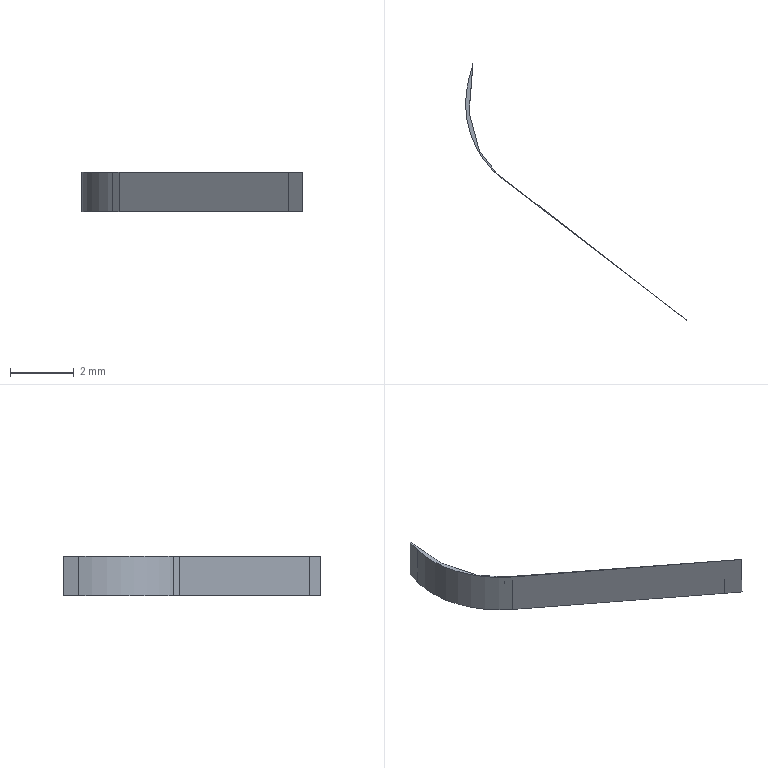Part | STEP file | gslz 2016.10.28-13_id1170_x_t | 1 solid | 10 faces | box 6.934 x 8.042 x 1.25 mm | volume 0.6004 mm3 | plane 9 | cylinder 1 | commonest cylinder face diameters 6 x1
STEP:
#1=CARTESIAN_POINT('',(0.,0.,0.));
#2=DIRECTION('',(0.,0.,1.));
#3=DIRECTION('',(1.,0.,0.));
#4=AXIS2_PLACEMENT_3D('',#1,#2,#3);
#5=CARTESIAN_POINT('',(-225.975,5.758,1.25));
#6=VERTEX_POINT('',#5);
#7=CARTESIAN_POINT('',(-225.435,5.068,1.25));
#8=VERTEX_POINT('',#7);
#9=CARTESIAN_POINT('',(-395.735,222.659,1.25));
#10=DIRECTION('',(0.6163,-0.7875,0.));
#11=VECTOR('',#10,1.);
#12=LINE('',#9,#11);
#13=CARTESIAN_POINT('',(-225.975,5.758,3.25));
#14=DIRECTION('',(0.7875,0.6163,0.));
#15=DIRECTION('',(-0.6163,0.7875,0.));
#16=AXIS2_PLACEMENT_3D('',#13,#14,#15);
#17=PLANE('',#16);
#18=CARTESIAN_POINT('',(275.435,-2.));
#19=DIRECTION('',(-1.,0.));
#20=VECTOR('',#19,1.);
#21=LINE('',#18,#20);
#22=(GEOMETRIC_REPRESENTATION_CONTEXT(2)PARAMETRIC_REPRESENTATION_CONTEXT()REPRESENTATION_CONTEXT('',''));
#23=DEFINITIONAL_REPRESENTATION('',(#21),#22);
#24=PCURVE('',#17,#23);
#25=CARTESIAN_POINT('',(-346.108,261.5,1.25));
#26=DIRECTION('',(0.,0.,-1.));
#27=DIRECTION('',(-1.,0.,0.));
#28=AXIS2_PLACEMENT_3D('',#25,#26,#27);
#29=PLANE('',#28);
#30=CARTESIAN_POINT('',(49.627,-38.841));
#31=DIRECTION('',(-0.6163,-0.7875));
#32=VECTOR('',#31,1.);
#33=LINE('',#30,#32);
#34=(GEOMETRIC_REPRESENTATION_CONTEXT(2)PARAMETRIC_REPRESENTATION_CONTEXT()REPRESENTATION_CONTEXT('',''));
#35=DEFINITIONAL_REPRESENTATION('',(#33),#34);
#36=PCURVE('',#29,#35);
#37=SURFACE_CURVE('',#12,(#24,#36),.PCURVE_S1.);
#38=EDGE_CURVE('',#6,#8,#37,.T.);
#39=ORIENTED_EDGE('',*,*,#38,.T.);
#40=CARTESIAN_POINT('',(-225.435,5.068,0.));
#41=VERTEX_POINT('',#40);
#42=CARTESIAN_POINT('',(-225.435,5.068,3.25));
#43=DIRECTION('',(0.,0.,1.));
#44=VECTOR('',#43,1.);
#45=LINE('',#42,#44);
#46=CARTESIAN_POINT('',(-0.8762,0.));
#47=DIRECTION('',(0.,1.));
#48=VECTOR('',#47,1.);
#49=LINE('',#46,#48);
#50=(GEOMETRIC_REPRESENTATION_CONTEXT(2)PARAMETRIC_REPRESENTATION_CONTEXT()REPRESENTATION_CONTEXT('',''));
#51=DEFINITIONAL_REPRESENTATION('',(#49),#50);
#52=PCURVE('',#17,#51);
#53=CARTESIAN_POINT('',(-225.435,5.068,3.25));
#54=DIRECTION('',(0.6121,0.7907,0.));
#55=DIRECTION('',(-0.7907,0.6121,0.));
#56=AXIS2_PLACEMENT_3D('',#53,#54,#55);
#57=PLANE('',#56);
#58=CARTESIAN_POINT('',(0.,0.));
#59=DIRECTION('',(0.,1.));
#60=VECTOR('',#59,1.);
#61=LINE('',#58,#60);
#62=(GEOMETRIC_REPRESENTATION_CONTEXT(2)PARAMETRIC_REPRESENTATION_CONTEXT()REPRESENTATION_CONTEXT('',''));
#63=DEFINITIONAL_REPRESENTATION('',(#61),#62);
#64=PCURVE('',#57,#63);
#65=SURFACE_CURVE('',#45,(#52,#64),.PCURVE_S1.);
#66=EDGE_CURVE('',#41,#8,#65,.T.);
#67=ORIENTED_EDGE('',*,*,#66,.F.);
#68=CARTESIAN_POINT('',(-225.975,5.758,0.));
#69=VERTEX_POINT('',#68);
#70=CARTESIAN_POINT('',(-225.975,5.758,0.));
#71=DIRECTION('',(0.6163,-0.7875,0.));
#72=VECTOR('',#71,1.);
#73=LINE('',#70,#72);
#74=CARTESIAN_POINT('',(0.,-3.25));
#75=DIRECTION('',(-1.,0.));
#76=VECTOR('',#75,1.);
#77=LINE('',#74,#76);
#78=(GEOMETRIC_REPRESENTATION_CONTEXT(2)PARAMETRIC_REPRESENTATION_CONTEXT()REPRESENTATION_CONTEXT('',''));
#79=DEFINITIONAL_REPRESENTATION('',(#77),#78);
#80=PCURVE('',#17,#79);
#81=CARTESIAN_POINT('',(-346.108,261.5,0.));
#82=DIRECTION('',(0.,0.,-1.));
#83=DIRECTION('',(-1.,0.,0.));
#84=AXIS2_PLACEMENT_3D('',#81,#82,#83);
#85=PLANE('',#84);
#86=CARTESIAN_POINT('',(-120.133,-255.742));
#87=DIRECTION('',(-0.6163,-0.7875));
#88=VECTOR('',#87,1.);
#89=LINE('',#86,#88);
#90=(GEOMETRIC_REPRESENTATION_CONTEXT(2)PARAMETRIC_REPRESENTATION_CONTEXT()REPRESENTATION_CONTEXT('',''));
#91=DEFINITIONAL_REPRESENTATION('',(#89),#90);
#92=PCURVE('',#85,#91);
#93=SURFACE_CURVE('',#73,(#80,#92),.PCURVE_S1.);
#94=EDGE_CURVE('',#69,#41,#93,.T.);
#95=ORIENTED_EDGE('',*,*,#94,.F.);
#96=CARTESIAN_POINT('',(-225.975,5.758,3.25));
#97=DIRECTION('',(0.,0.,1.));
#98=VECTOR('',#97,1.);
#99=LINE('',#96,#98);
#100=CARTESIAN_POINT('',(0.,0.));
#101=DIRECTION('',(0.,1.));
#102=VECTOR('',#101,1.);
#103=LINE('',#100,#102);
#104=(GEOMETRIC_REPRESENTATION_CONTEXT(2)PARAMETRIC_REPRESENTATION_CONTEXT()REPRESENTATION_CONTEXT('',''));
#105=DEFINITIONAL_REPRESENTATION('',(#103),#104);
#106=PCURVE('',#17,#105);
#107=CARTESIAN_POINT('',(-226.305,6.991,3.25));
#108=DIRECTION('',(0.966,0.2585,0.));
#109=DIRECTION('',(-0.2585,0.966,0.));
#110=AXIS2_PLACEMENT_3D('',#107,#108,#109);
#111=PLANE('',#110);
#112=CARTESIAN_POINT('',(-1.276,0.));
#113=DIRECTION('',(0.,1.));
#114=VECTOR('',#113,1.);
#115=LINE('',#112,#114);
#116=(GEOMETRIC_REPRESENTATION_CONTEXT(2)PARAMETRIC_REPRESENTATION_CONTEXT()REPRESENTATION_CONTEXT('',''));
#117=DEFINITIONAL_REPRESENTATION('',(#115),#116);
#118=PCURVE('',#111,#117);
#119=SURFACE_CURVE('',#99,(#106,#118),.PCURVE_S1.);
#120=EDGE_CURVE('',#69,#6,#119,.T.);
#121=ORIENTED_EDGE('',*,*,#120,.T.);
#122=EDGE_LOOP('',(#39,#67,#95,#121));
#123=FACE_BOUND('',#122,.T.);
#124=ADVANCED_FACE('',(#123),#17,.T.);
#125=CARTESIAN_POINT('',(-226.305,6.991,1.25));
#126=VERTEX_POINT('',#125);
#127=CARTESIAN_POINT('',(-297.867,274.409,1.25));
#128=DIRECTION('',(0.2585,-0.966,0.));
#129=VECTOR('',#128,1.);
#130=LINE('',#127,#129);
#131=CARTESIAN_POINT('',(276.828,-2.));
#132=DIRECTION('',(-1.,0.));
#133=VECTOR('',#132,1.);
#134=LINE('',#131,#133);
#135=(GEOMETRIC_REPRESENTATION_CONTEXT(2)PARAMETRIC_REPRESENTATION_CONTEXT()REPRESENTATION_CONTEXT('',''));
#136=DEFINITIONAL_REPRESENTATION('',(#134),#135);
#137=PCURVE('',#111,#136);
#138=CARTESIAN_POINT('',(-48.241,12.909));
#139=DIRECTION('',(-0.2585,-0.966));
#140=VECTOR('',#139,1.);
#141=LINE('',#138,#140);
#142=(GEOMETRIC_REPRESENTATION_CONTEXT(2)PARAMETRIC_REPRESENTATION_CONTEXT()REPRESENTATION_CONTEXT('',''));
#143=DEFINITIONAL_REPRESENTATION('',(#141),#142);
#144=PCURVE('',#29,#143);
#145=SURFACE_CURVE('',#130,(#137,#144),.PCURVE_S1.);
#146=EDGE_CURVE('',#126,#6,#145,.T.);
#147=ORIENTED_EDGE('',*,*,#146,.T.);
#148=ORIENTED_EDGE('',*,*,#120,.F.);
#149=CARTESIAN_POINT('',(-226.305,6.991,0.));
#150=VERTEX_POINT('',#149);
#151=CARTESIAN_POINT('',(-226.305,6.991,0.));
#152=DIRECTION('',(0.2585,-0.966,0.));
#153=VECTOR('',#152,1.);
#154=LINE('',#151,#153);
#155=CARTESIAN_POINT('',(0.,-3.25));
#156=DIRECTION('',(-1.,0.));
#157=VECTOR('',#156,1.);
#158=LINE('',#155,#157);
#159=(GEOMETRIC_REPRESENTATION_CONTEXT(2)PARAMETRIC_REPRESENTATION_CONTEXT()REPRESENTATION_CONTEXT('',''));
#160=DEFINITIONAL_REPRESENTATION('',(#158),#159);
#161=PCURVE('',#111,#160);
#162=CARTESIAN_POINT('',(-119.803,-254.509));
#163=DIRECTION('',(-0.2585,-0.966));
#164=VECTOR('',#163,1.);
#165=LINE('',#162,#164);
#166=(GEOMETRIC_REPRESENTATION_CONTEXT(2)PARAMETRIC_REPRESENTATION_CONTEXT()REPRESENTATION_CONTEXT('',''));
#167=DEFINITIONAL_REPRESENTATION('',(#165),#166);
#168=PCURVE('',#85,#167);
#169=SURFACE_CURVE('',#154,(#161,#168),.PCURVE_S1.);
#170=EDGE_CURVE('',#150,#69,#169,.T.);
#171=ORIENTED_EDGE('',*,*,#170,.F.);
#172=CARTESIAN_POINT('',(-226.305,6.991,3.25));
#173=DIRECTION('',(0.,0.,1.));
#174=VECTOR('',#173,1.);
#175=LINE('',#172,#174);
#176=CARTESIAN_POINT('',(0.,0.));
#177=DIRECTION('',(0.,1.));
#178=VECTOR('',#177,1.);
#179=LINE('',#176,#178);
#180=(GEOMETRIC_REPRESENTATION_CONTEXT(2)PARAMETRIC_REPRESENTATION_CONTEXT()REPRESENTATION_CONTEXT('',''));
#181=DEFINITIONAL_REPRESENTATION('',(#179),#180);
#182=PCURVE('',#111,#181);
#183=CARTESIAN_POINT('',(-226.185,8.501,3.25));
#184=DIRECTION('',(0.9969,-0.07922,0.));
#185=DIRECTION('',(0.07922,0.9969,0.));
#186=AXIS2_PLACEMENT_3D('',#183,#184,#185);
#187=PLANE('',#186);
#188=CARTESIAN_POINT('',(-1.515,0.));
#189=DIRECTION('',(0.,1.));
#190=VECTOR('',#189,1.);
#191=LINE('',#188,#190);
#192=(GEOMETRIC_REPRESENTATION_CONTEXT(2)PARAMETRIC_REPRESENTATION_CONTEXT()REPRESENTATION_CONTEXT('',''));
#193=DEFINITIONAL_REPRESENTATION('',(#191),#192);
#194=PCURVE('',#187,#193);
#195=SURFACE_CURVE('',#175,(#182,#194),.PCURVE_S1.);
#196=EDGE_CURVE('',#150,#126,#195,.T.);
#197=ORIENTED_EDGE('',*,*,#196,.T.);
#198=EDGE_LOOP('',(#147,#148,#171,#197));
#199=FACE_BOUND('',#198,.T.);
#200=ADVANCED_FACE('',(#199),#111,.T.);
#201=CARTESIAN_POINT('',(-219.911,0.7917,1.25));
#202=VERTEX_POINT('',#201);
#203=CARTESIAN_POINT('',(-425.016,159.57,1.25));
#204=DIRECTION('',(0.7907,-0.6121,0.));
#205=VECTOR('',#204,1.);
#206=LINE('',#203,#205);
#207=CARTESIAN_POINT('',(252.395,-2.));
#208=DIRECTION('',(-1.,0.));
#209=VECTOR('',#208,1.);
#210=LINE('',#207,#209);
#211=(GEOMETRIC_REPRESENTATION_CONTEXT(2)PARAMETRIC_REPRESENTATION_CONTEXT()REPRESENTATION_CONTEXT('',''));
#212=DEFINITIONAL_REPRESENTATION('',(#210),#211);
#213=PCURVE('',#57,#212);
#214=CARTESIAN_POINT('',(78.908,-101.93));
#215=DIRECTION('',(-0.7907,-0.6121));
#216=VECTOR('',#215,1.);
#217=LINE('',#214,#216);
#218=(GEOMETRIC_REPRESENTATION_CONTEXT(2)PARAMETRIC_REPRESENTATION_CONTEXT()REPRESENTATION_CONTEXT('',''));
#219=DEFINITIONAL_REPRESENTATION('',(#217),#218);
#220=PCURVE('',#29,#219);
#221=SURFACE_CURVE('',#206,(#213,#220),.PCURVE_S1.);
#222=EDGE_CURVE('',#8,#202,#221,.T.);
#223=ORIENTED_EDGE('',*,*,#222,.T.);
#224=CARTESIAN_POINT('',(-219.911,0.7917,0.));
#225=VERTEX_POINT('',#224);
#226=CARTESIAN_POINT('',(-219.911,0.7917,3.25));
#227=DIRECTION('',(0.,0.,1.));
#228=VECTOR('',#227,1.);
#229=LINE('',#226,#228);
#230=CARTESIAN_POINT('',(-6.985,0.));
#231=DIRECTION('',(0.,1.));
#232=VECTOR('',#231,1.);
#233=LINE('',#230,#232);
#234=(GEOMETRIC_REPRESENTATION_CONTEXT(2)PARAMETRIC_REPRESENTATION_CONTEXT()REPRESENTATION_CONTEXT('',''));
#235=DEFINITIONAL_REPRESENTATION('',(#233),#234);
#236=PCURVE('',#57,#235);
#237=CARTESIAN_POINT('',(-219.911,0.7917,3.25));
#238=DIRECTION('',(0.6121,0.7908,0.));
#239=DIRECTION('',(-0.7908,0.6121,0.));
#240=AXIS2_PLACEMENT_3D('',#237,#238,#239);
#241=PLANE('',#240);
#242=CARTESIAN_POINT('',(0.,0.));
#243=DIRECTION('',(0.,1.));
#244=VECTOR('',#243,1.);
#245=LINE('',#242,#244);
#246=(GEOMETRIC_REPRESENTATION_CONTEXT(2)PARAMETRIC_REPRESENTATION_CONTEXT()REPRESENTATION_CONTEXT('',''));
#247=DEFINITIONAL_REPRESENTATION('',(#245),#246);
#248=PCURVE('',#241,#247);
#249=SURFACE_CURVE('',#229,(#236,#248),.PCURVE_S1.);
#250=EDGE_CURVE('',#225,#202,#249,.T.);
#251=ORIENTED_EDGE('',*,*,#250,.F.);
#252=CARTESIAN_POINT('',(-225.435,5.068,0.));
#253=DIRECTION('',(0.7907,-0.6121,0.));
#254=VECTOR('',#253,1.);
#255=LINE('',#252,#254);
#256=CARTESIAN_POINT('',(0.,-3.25));
#257=DIRECTION('',(-1.,0.));
#258=VECTOR('',#257,1.);
#259=LINE('',#256,#258);
#260=(GEOMETRIC_REPRESENTATION_CONTEXT(2)PARAMETRIC_REPRESENTATION_CONTEXT()REPRESENTATION_CONTEXT('',''));
#261=DEFINITIONAL_REPRESENTATION('',(#259),#260);
#262=PCURVE('',#57,#261);
#263=CARTESIAN_POINT('',(-120.673,-256.432));
#264=DIRECTION('',(-0.7907,-0.6121));
#265=VECTOR('',#264,1.);
#266=LINE('',#263,#265);
#267=(GEOMETRIC_REPRESENTATION_CONTEXT(2)PARAMETRIC_REPRESENTATION_CONTEXT()REPRESENTATION_CONTEXT('',''));
#268=DEFINITIONAL_REPRESENTATION('',(#266),#267);
#269=PCURVE('',#85,#268);
#270=SURFACE_CURVE('',#255,(#262,#269),.PCURVE_S1.);
#271=EDGE_CURVE('',#41,#225,#270,.T.);
#272=ORIENTED_EDGE('',*,*,#271,.F.);
#273=ORIENTED_EDGE('',*,*,#66,.T.);
#274=EDGE_LOOP('',(#223,#251,#272,#273));
#275=FACE_BOUND('',#274,.T.);
#276=ADVANCED_FACE('',(#275),#57,.T.);
#277=CARTESIAN_POINT('',(-219.481,0.4587,1.25));
#278=VERTEX_POINT('',#277);
#279=CARTESIAN_POINT('',(-425.016,159.568,1.25));
#280=DIRECTION('',(0.7908,-0.6121,0.));
#281=VECTOR('',#280,1.);
#282=LINE('',#279,#281);
#283=CARTESIAN_POINT('',(259.38,-2.));
#284=DIRECTION('',(-1.,0.));
#285=VECTOR('',#284,1.);
#286=LINE('',#283,#285);
#287=(GEOMETRIC_REPRESENTATION_CONTEXT(2)PARAMETRIC_REPRESENTATION_CONTEXT()REPRESENTATION_CONTEXT('',''));
#288=DEFINITIONAL_REPRESENTATION('',(#286),#287);
#289=PCURVE('',#241,#288);
#290=CARTESIAN_POINT('',(78.908,-101.932));
#291=DIRECTION('',(-0.7908,-0.6121));
#292=VECTOR('',#291,1.);
#293=LINE('',#290,#292);
#294=(GEOMETRIC_REPRESENTATION_CONTEXT(2)PARAMETRIC_REPRESENTATION_CONTEXT()REPRESENTATION_CONTEXT('',''));
#295=DEFINITIONAL_REPRESENTATION('',(#293),#294);
#296=PCURVE('',#29,#295);
#297=SURFACE_CURVE('',#282,(#289,#296),.PCURVE_S1.);
#298=EDGE_CURVE('',#202,#278,#297,.T.);
#299=ORIENTED_EDGE('',*,*,#298,.T.);
#300=CARTESIAN_POINT('',(-219.481,0.4587,0.));
#301=VERTEX_POINT('',#300);
#302=CARTESIAN_POINT('',(-219.481,0.4587,3.25));
#303=DIRECTION('',(0.000000009,-0.000000007,-1.));
#304=VECTOR('',#303,1.);
#305=LINE('',#302,#304);
#306=CARTESIAN_POINT('',(-0.544,0.000000006));
#307=DIRECTION('',(-0.000000012,-1.));
#308=VECTOR('',#307,1.);
#309=LINE('',#306,#308);
#310=(GEOMETRIC_REPRESENTATION_CONTEXT(2)PARAMETRIC_REPRESENTATION_CONTEXT()REPRESENTATION_CONTEXT('',''));
#311=DEFINITIONAL_REPRESENTATION('',(#309),#310);
#312=PCURVE('',#241,#311);
#313=CARTESIAN_POINT('',(-208.094,-8.268,1.25));
#314=DIRECTION('',(-0.6083,-0.7937,0.));
#315=DIRECTION('',(-0.7924,0.6073,-0.05661));
#316=AXIS2_PLACEMENT_3D('',#313,#314,#315);
#317=PLANE('',#316);
#318=CARTESIAN_POINT('',(14.21,-2.809));
#319=DIRECTION('',(0.05661,0.9984));
#320=VECTOR('',#319,1.);
#321=LINE('',#318,#320);
#322=(GEOMETRIC_REPRESENTATION_CONTEXT(2)PARAMETRIC_REPRESENTATION_CONTEXT()REPRESENTATION_CONTEXT('',''));
#323=DEFINITIONAL_REPRESENTATION('',(#321),#322);
#324=PCURVE('',#317,#323);
#325=SURFACE_CURVE('',#305,(#312,#324),.PCURVE_S1.);
#326=EDGE_CURVE('',#278,#301,#325,.T.);
#327=ORIENTED_EDGE('',*,*,#326,.T.);
#328=CARTESIAN_POINT('',(-219.911,0.7917,0.));
#329=DIRECTION('',(0.7908,-0.6121,0.));
#330=VECTOR('',#329,1.);
#331=LINE('',#328,#330);
#332=CARTESIAN_POINT('',(0.,-3.25));
#333=DIRECTION('',(-1.,0.));
#334=VECTOR('',#333,1.);
#335=LINE('',#332,#334);
#336=(GEOMETRIC_REPRESENTATION_CONTEXT(2)PARAMETRIC_REPRESENTATION_CONTEXT()REPRESENTATION_CONTEXT('',''));
#337=DEFINITIONAL_REPRESENTATION('',(#335),#336);
#338=PCURVE('',#241,#337);
#339=CARTESIAN_POINT('',(-126.197,-260.708));
#340=DIRECTION('',(-0.7908,-0.6121));
#341=VECTOR('',#340,1.);
#342=LINE('',#339,#341);
#343=(GEOMETRIC_REPRESENTATION_CONTEXT(2)PARAMETRIC_REPRESENTATION_CONTEXT()REPRESENTATION_CONTEXT('',''));
#344=DEFINITIONAL_REPRESENTATION('',(#342),#343);
#345=PCURVE('',#85,#344);
#346=SURFACE_CURVE('',#331,(#338,#345),.PCURVE_S1.);
#347=EDGE_CURVE('',#225,#301,#346,.T.);
#348=ORIENTED_EDGE('',*,*,#347,.F.);
#349=ORIENTED_EDGE('',*,*,#250,.T.);
#350=EDGE_LOOP('',(#299,#327,#348,#349));
#351=FACE_BOUND('',#350,.T.);
#352=ADVANCED_FACE('',(#351),#241,.T.);
#353=CARTESIAN_POINT('',(-226.185,8.501,-0.000001375));
#354=VERTEX_POINT('',#353);
#355=CARTESIAN_POINT('',(-226.31,8.042,-0.000001375));
#356=VERTEX_POINT('',#355);
#357=CARTESIAN_POINT('',(-258.27,-109.301,-0.000001364));
#358=DIRECTION('',(-0.2628,-0.9649,0.));
#359=VECTOR('',#358,1.);
#360=LINE('',#357,#359);
#361=CARTESIAN_POINT('',(-87.838,-370.801));
#362=DIRECTION('',(0.2628,-0.9649));
#363=VECTOR('',#362,1.);
#364=LINE('',#361,#363);
#365=(GEOMETRIC_REPRESENTATION_CONTEXT(2)PARAMETRIC_REPRESENTATION_CONTEXT()REPRESENTATION_CONTEXT('',''));
#366=DEFINITIONAL_REPRESENTATION('',(#364),#365);
#367=PCURVE('',#85,#366);
#368=CARTESIAN_POINT('',(-224.715,13.898,3.25));
#369=DIRECTION('',(0.9649,-0.2628,0.));
#370=DIRECTION('',(0.2628,0.9649,0.));
#371=AXIS2_PLACEMENT_3D('',#368,#369,#370);
#372=PLANE('',#371);
#373=CARTESIAN_POINT('',(-127.686,-3.25));
#374=DIRECTION('',(-1.,0.));
#375=VECTOR('',#374,1.);
#376=LINE('',#373,#375);
#377=(GEOMETRIC_REPRESENTATION_CONTEXT(2)PARAMETRIC_REPRESENTATION_CONTEXT()REPRESENTATION_CONTEXT('',''));
#378=DEFINITIONAL_REPRESENTATION('',(#376),#377);
#379=PCURVE('',#372,#378);
#380=SURFACE_CURVE('',#360,(#367,#379),.PCURVE_S1.);
#381=EDGE_CURVE('',#354,#356,#380,.T.);
#382=ORIENTED_EDGE('',*,*,#381,.F.);
#383=CARTESIAN_POINT('',(-226.185,8.501,0.));
#384=DIRECTION('',(-0.07922,-0.9969,0.));
#385=VECTOR('',#384,1.);
#386=LINE('',#383,#385);
#387=CARTESIAN_POINT('',(-119.923,-252.999));
#388=DIRECTION('',(0.07922,-0.9969));
#389=VECTOR('',#388,1.);
#390=LINE('',#387,#389);
#391=(GEOMETRIC_REPRESENTATION_CONTEXT(2)PARAMETRIC_REPRESENTATION_CONTEXT()REPRESENTATION_CONTEXT('',''));
#392=DEFINITIONAL_REPRESENTATION('',(#390),#391);
#393=PCURVE('',#85,#392);
#394=CARTESIAN_POINT('',(0.,-3.25));
#395=DIRECTION('',(-1.,0.));
#396=VECTOR('',#395,1.);
#397=LINE('',#394,#396);
#398=(GEOMETRIC_REPRESENTATION_CONTEXT(2)PARAMETRIC_REPRESENTATION_CONTEXT()REPRESENTATION_CONTEXT('',''));
#399=DEFINITIONAL_REPRESENTATION('',(#397),#398);
#400=PCURVE('',#187,#399);
#401=SURFACE_CURVE('',#386,(#393,#400),.PCURVE_S1.);
#402=EDGE_CURVE('',#354,#150,#401,.T.);
#403=ORIENTED_EDGE('',*,*,#402,.T.);
#404=ORIENTED_EDGE('',*,*,#170,.T.);
#405=ORIENTED_EDGE('',*,*,#94,.T.);
#406=ORIENTED_EDGE('',*,*,#271,.T.);
#407=ORIENTED_EDGE('',*,*,#347,.T.);
#408=CARTESIAN_POINT('',(-225.24,4.872,-0.000001374));
#409=VERTEX_POINT('',#408);
#410=CARTESIAN_POINT('',(-229.545,8.172,-0.000001375));
#411=CARTESIAN_POINT('',(-226.747,6.027,-0.000001374));
#412=CARTESIAN_POINT('',(-225.232,4.866,-0.000001374));
#413=CARTESIAN_POINT('',(-208.094,-8.268,-0.000001372));
#414=CARTESIAN_POINT('',(-205.296,-10.413,-0.000001372));
#415=B_SPLINE_CURVE_WITH_KNOTS('',1,(#410,#411,#412,#413,#414),.UNSPECIFIED.,.F.,.F.,(2,1,1,1,2),(0.,0.1154,0.1779,0.8846,1.),.UNSPECIFIED.);
#416=CARTESIAN_POINT('',(-116.563,-253.328));
#417=CARTESIAN_POINT('',(-119.361,-255.473));
#418=CARTESIAN_POINT('',(-120.876,-256.634));
#419=CARTESIAN_POINT('',(-138.014,-269.768));
#420=CARTESIAN_POINT('',(-140.812,-271.913));
#421=B_SPLINE_CURVE_WITH_KNOTS('',1,(#416,#417,#418,#419,#420),.UNSPECIFIED.,.F.,.F.,(2,1,1,1,2),(0.,0.1154,0.1779,0.8846,1.),.UNSPECIFIED.);
#422=(GEOMETRIC_REPRESENTATION_CONTEXT(2)PARAMETRIC_REPRESENTATION_CONTEXT()REPRESENTATION_CONTEXT('',''));
#423=DEFINITIONAL_REPRESENTATION('',(#421),#422);
#424=PCURVE('',#85,#423);
#425=CARTESIAN_POINT('',(27.053,-0.2818));
#426=CARTESIAN_POINT('',(23.534,-0.08229));
#427=CARTESIAN_POINT('',(21.628,0.02575));
#428=CARTESIAN_POINT('',(0.07076,1.248));
#429=CARTESIAN_POINT('',(-3.449,1.448));
#430=B_SPLINE_CURVE_WITH_KNOTS('',1,(#425,#426,#427,#428,#429),.UNSPECIFIED.,.F.,.F.,(2,1,1,1,2),(0.,0.1154,0.1779,0.8846,1.),.UNSPECIFIED.);
#431=(GEOMETRIC_REPRESENTATION_CONTEXT(2)PARAMETRIC_REPRESENTATION_CONTEXT()REPRESENTATION_CONTEXT('',''));
#432=DEFINITIONAL_REPRESENTATION('',(#430),#431);
#433=PCURVE('',#317,#432);
#434=SURFACE_CURVE('',#415,(#424,#433),.PCURVE_S1.);
#435=EDGE_CURVE('',#409,#301,#434,.T.);
#436=ORIENTED_EDGE('',*,*,#435,.F.);
#437=CARTESIAN_POINT('',(-223.415,7.254,-0.000001375));
#438=DIRECTION('',(0.,0.,1.));
#439=DIRECTION('',(0.,1.,0.));
#440=AXIS2_PLACEMENT_3D('',#437,#438,#439);
#441=CIRCLE('',#440,3.);
#442=CARTESIAN_POINT('',(-122.693,-251.246));
#443=CARTESIAN_POINT('',(-117.497,-251.246));
#444=CARTESIAN_POINT('',(-120.095,-255.746));
#445=CARTESIAN_POINT('',(-122.693,-260.246));
#446=CARTESIAN_POINT('',(-125.291,-255.746));
#447=CARTESIAN_POINT('',(-127.889,-251.246));
#448=CARTESIAN_POINT('',(-122.693,-251.246));
#449=(BOUNDED_CURVE()B_SPLINE_CURVE(2,(#442,#443,#444,#445,#446,#447,#448),.UNSPECIFIED.,.T.,.F.)B_SPLINE_CURVE_WITH_KNOTS((1,2,2,2,2,1),(-2.094,0.,2.094,4.189,6.283,8.378),.UNSPECIFIED.)CURVE()GEOMETRIC_REPRESENTATION_ITEM()RATIONAL_B_SPLINE_CURVE((1.,0.5,1.,0.5,1.,0.5,1.))REPRESENTATION_ITEM(''));
#450=(GEOMETRIC_REPRESENTATION_CONTEXT(2)PARAMETRIC_REPRESENTATION_CONTEXT()REPRESENTATION_CONTEXT('',''));
#451=DEFINITIONAL_REPRESENTATION('',(#449),#450);
#452=PCURVE('',#85,#451);
#453=CARTESIAN_POINT('',(-223.415,7.254,3.25));
#454=DIRECTION('',(0.,0.,-1.));
#455=DIRECTION('',(0.,1.,0.));
#456=AXIS2_PLACEMENT_3D('',#453,#454,#455);
#457=CYLINDRICAL_SURFACE('',#456,3.);
#458=CARTESIAN_POINT('',(6.283,3.25));
#459=DIRECTION('',(-1.,0.));
#460=VECTOR('',#459,1.);
#461=LINE('',#458,#460);
#462=(GEOMETRIC_REPRESENTATION_CONTEXT(2)PARAMETRIC_REPRESENTATION_CONTEXT()REPRESENTATION_CONTEXT('',''));
#463=DEFINITIONAL_REPRESENTATION('',(#461),#462);
#464=PCURVE('',#457,#463);
#465=SURFACE_CURVE('',#441,(#452,#464),.PCURVE_S1.);
#466=EDGE_CURVE('',#356,#409,#465,.T.);
#467=ORIENTED_EDGE('',*,*,#466,.F.);
#468=EDGE_LOOP('',(#382,#403,#404,#405,#406,#407,#436,#467));
#469=FACE_BOUND('',#468,.T.);
#470=ADVANCED_FACE('',(#469),#85,.T.);
#471=CARTESIAN_POINT('',(-226.185,8.501,1.25));
#472=VERTEX_POINT('',#471);
#473=CARTESIAN_POINT('',(-206.958,250.442,1.25));
#474=DIRECTION('',(-0.07922,-0.9969,0.));
#475=VECTOR('',#474,1.);
#476=LINE('',#473,#475);
#477=CARTESIAN_POINT('',(242.704,-2.));
#478=DIRECTION('',(-1.,0.));
#479=VECTOR('',#478,1.);
#480=LINE('',#477,#479);
#481=(GEOMETRIC_REPRESENTATION_CONTEXT(2)PARAMETRIC_REPRESENTATION_CONTEXT()REPRESENTATION_CONTEXT('',''));
#482=DEFINITIONAL_REPRESENTATION('',(#480),#481);
#483=PCURVE('',#187,#482);
#484=CARTESIAN_POINT('',(-139.15,-11.058));
#485=DIRECTION('',(0.07922,-0.9969));
#486=VECTOR('',#485,1.);
#487=LINE('',#484,#486);
#488=(GEOMETRIC_REPRESENTATION_CONTEXT(2)PARAMETRIC_REPRESENTATION_CONTEXT()REPRESENTATION_CONTEXT('',''));
#489=DEFINITIONAL_REPRESENTATION('',(#487),#488);
#490=PCURVE('',#29,#489);
#491=SURFACE_CURVE('',#476,(#483,#490),.PCURVE_S1.);
#492=EDGE_CURVE('',#472,#126,#491,.T.);
#493=ORIENTED_EDGE('',*,*,#492,.T.);
#494=ORIENTED_EDGE('',*,*,#196,.F.);
#495=ORIENTED_EDGE('',*,*,#402,.F.);
#496=CARTESIAN_POINT('',(-226.185,8.501,3.25));
#497=DIRECTION('',(0.,0.,1.));
#498=VECTOR('',#497,1.);
#499=LINE('',#496,#498);
#500=CARTESIAN_POINT('',(0.,0.));
#501=DIRECTION('',(0.,1.));
#502=VECTOR('',#501,1.);
#503=LINE('',#500,#502);
#504=(GEOMETRIC_REPRESENTATION_CONTEXT(2)PARAMETRIC_REPRESENTATION_CONTEXT()REPRESENTATION_CONTEXT('',''));
#505=DEFINITIONAL_REPRESENTATION('',(#503),#504);
#506=PCURVE('',#187,#505);
#507=CARTESIAN_POINT('',(-5.594,0.));
#508=DIRECTION('',(0.,1.));
#509=VECTOR('',#508,1.);
#510=LINE('',#507,#509);
#511=(GEOMETRIC_REPRESENTATION_CONTEXT(2)PARAMETRIC_REPRESENTATION_CONTEXT()REPRESENTATION_CONTEXT('',''));
#512=DEFINITIONAL_REPRESENTATION('',(#510),#511);
#513=PCURVE('',#372,#512);
#514=SURFACE_CURVE('',#499,(#506,#513),.PCURVE_S1.);
#515=EDGE_CURVE('',#354,#472,#514,.T.);
#516=ORIENTED_EDGE('',*,*,#515,.T.);
#517=EDGE_LOOP('',(#493,#494,#495,#516));
#518=FACE_BOUND('',#517,.T.);
#519=ADVANCED_FACE('',(#518),#187,.T.);
#520=CARTESIAN_POINT('',(-226.31,8.042,1.25));
#521=VERTEX_POINT('',#520);
#522=CARTESIAN_POINT('',(-258.27,-109.301,1.25));
#523=DIRECTION('',(-0.2628,-0.9649,0.));
#524=VECTOR('',#523,1.);
#525=LINE('',#522,#524);
#526=CARTESIAN_POINT('',(-87.838,-370.801));
#527=DIRECTION('',(0.2628,-0.9649));
#528=VECTOR('',#527,1.);
#529=LINE('',#526,#528);
#530=(GEOMETRIC_REPRESENTATION_CONTEXT(2)PARAMETRIC_REPRESENTATION_CONTEXT()REPRESENTATION_CONTEXT('',''));
#531=DEFINITIONAL_REPRESENTATION('',(#529),#530);
#532=PCURVE('',#29,#531);
#533=CARTESIAN_POINT('',(-127.686,-2.));
#534=DIRECTION('',(-1.,0.));
#535=VECTOR('',#534,1.);
#536=LINE('',#533,#535);
#537=(GEOMETRIC_REPRESENTATION_CONTEXT(2)PARAMETRIC_REPRESENTATION_CONTEXT()REPRESENTATION_CONTEXT('',''));
#538=DEFINITIONAL_REPRESENTATION('',(#536),#537);
#539=PCURVE('',#372,#538);
#540=SURFACE_CURVE('',#525,(#532,#539),.PCURVE_S1.);
#541=EDGE_CURVE('',#472,#521,#540,.T.);
#542=ORIENTED_EDGE('',*,*,#541,.F.);
#543=ORIENTED_EDGE('',*,*,#492,.T.);
#544=ORIENTED_EDGE('',*,*,#146,.T.);
#545=ORIENTED_EDGE('',*,*,#38,.T.);
#546=ORIENTED_EDGE('',*,*,#222,.T.);
#547=ORIENTED_EDGE('',*,*,#298,.T.);
#548=CARTESIAN_POINT('',(-225.24,4.872,1.25));
#549=VERTEX_POINT('',#548);
#550=CARTESIAN_POINT('',(-229.545,8.172,1.25));
#551=CARTESIAN_POINT('',(-226.747,6.027,1.25));
#552=CARTESIAN_POINT('',(-225.232,4.866,1.25));
#553=CARTESIAN_POINT('',(-208.094,-8.268,1.25));
#554=CARTESIAN_POINT('',(-205.296,-10.413,1.25));
#555=B_SPLINE_CURVE_WITH_KNOTS('',1,(#550,#551,#552,#553,#554),.UNSPECIFIED.,.F.,.F.,(2,1,1,1,2),(0.,0.1154,0.1779,0.8846,1.),.UNSPECIFIED.);
#556=CARTESIAN_POINT('',(-116.563,-253.328));
#557=CARTESIAN_POINT('',(-119.361,-255.473));
#558=CARTESIAN_POINT('',(-120.876,-256.634));
#559=CARTESIAN_POINT('',(-138.014,-269.768));
#560=CARTESIAN_POINT('',(-140.812,-271.913));
#561=B_SPLINE_CURVE_WITH_KNOTS('',1,(#556,#557,#558,#559,#560),.UNSPECIFIED.,.F.,.F.,(2,1,1,1,2),(0.,0.1154,0.1779,0.8846,1.),.UNSPECIFIED.);
#562=(GEOMETRIC_REPRESENTATION_CONTEXT(2)PARAMETRIC_REPRESENTATION_CONTEXT()REPRESENTATION_CONTEXT('',''));
#563=DEFINITIONAL_REPRESENTATION('',(#561),#562);
#564=PCURVE('',#29,#563);
#565=CARTESIAN_POINT('',(26.982,-1.53));
#566=CARTESIAN_POINT('',(23.463,-1.33));
#567=CARTESIAN_POINT('',(21.557,-1.222));
#568=CARTESIAN_POINT('',(0.,0.));
#569=CARTESIAN_POINT('',(-3.519,0.1995));
#570=B_SPLINE_CURVE_WITH_KNOTS('',1,(#565,#566,#567,#568,#569),.UNSPECIFIED.,.F.,.F.,(2,1,1,1,2),(0.,0.1154,0.1779,0.8846,1.),.UNSPECIFIED.);
#571=(GEOMETRIC_REPRESENTATION_CONTEXT(2)PARAMETRIC_REPRESENTATION_CONTEXT()REPRESENTATION_CONTEXT('',''));
#572=DEFINITIONAL_REPRESENTATION('',(#570),#571);
#573=PCURVE('',#317,#572);
#574=SURFACE_CURVE('',#555,(#564,#573),.PCURVE_S1.);
#575=EDGE_CURVE('',#549,#278,#574,.T.);
#576=ORIENTED_EDGE('',*,*,#575,.F.);
#577=CARTESIAN_POINT('',(-223.415,7.254,1.25));
#578=DIRECTION('',(0.,0.,-1.));
#579=DIRECTION('',(0.,1.,0.));
#580=AXIS2_PLACEMENT_3D('',#577,#578,#579);
#581=CIRCLE('',#580,3.);
#582=CARTESIAN_POINT('',(-122.693,-254.246));
#583=DIRECTION('',(0.,1.));
#584=AXIS2_PLACEMENT_2D('',#582,#583);
#585=CIRCLE('',#584,3.);
#586=(GEOMETRIC_REPRESENTATION_CONTEXT(2)PARAMETRIC_REPRESENTATION_CONTEXT()REPRESENTATION_CONTEXT('',''));
#587=DEFINITIONAL_REPRESENTATION('',(#585),#586);
#588=PCURVE('',#29,#587);
#589=CARTESIAN_POINT('',(0.,2.));
#590=DIRECTION('',(1.,0.));
#591=VECTOR('',#590,1.);
#592=LINE('',#589,#591);
#593=(GEOMETRIC_REPRESENTATION_CONTEXT(2)PARAMETRIC_REPRESENTATION_CONTEXT()REPRESENTATION_CONTEXT('',''));
#594=DEFINITIONAL_REPRESENTATION('',(#592),#593);
#595=PCURVE('',#457,#594);
#596=SURFACE_CURVE('',#581,(#588,#595),.PCURVE_S1.);
#597=EDGE_CURVE('',#549,#521,#596,.T.);
#598=ORIENTED_EDGE('',*,*,#597,.T.);
#599=EDGE_LOOP('',(#542,#543,#544,#545,#546,#547,#576,#598));
#600=FACE_BOUND('',#599,.F.);
#601=ADVANCED_FACE('',(#600),#29,.F.);
#602=ORIENTED_EDGE('',*,*,#575,.F.);
#603=CARTESIAN_POINT('',(-225.24,4.872,1.25));
#604=DIRECTION('',(0.,0.,-1.));
#605=VECTOR('',#604,1.);
#606=LINE('',#603,#605);
#607=CARTESIAN_POINT('',(21.568,-1.223));
#608=DIRECTION('',(0.05661,0.9984));
#609=VECTOR('',#608,1.);
#610=LINE('',#607,#609);
#611=(GEOMETRIC_REPRESENTATION_CONTEXT(2)PARAMETRIC_REPRESENTATION_CONTEXT()REPRESENTATION_CONTEXT('',''));
#612=DEFINITIONAL_REPRESENTATION('',(#610),#611);
#613=PCURVE('',#317,#612);
#614=CARTESIAN_POINT('',(3.796,2.));
#615=DIRECTION('',(0.,1.));
#616=VECTOR('',#615,1.);
#617=LINE('',#614,#616);
#618=(GEOMETRIC_REPRESENTATION_CONTEXT(2)PARAMETRIC_REPRESENTATION_CONTEXT()REPRESENTATION_CONTEXT('',''));
#619=DEFINITIONAL_REPRESENTATION('',(#617),#618);
#620=PCURVE('',#457,#619);
#621=SURFACE_CURVE('',#606,(#613,#620),.PCURVE_S1.);
#622=EDGE_CURVE('',#549,#409,#621,.T.);
#623=ORIENTED_EDGE('',*,*,#622,.T.);
#624=ORIENTED_EDGE('',*,*,#435,.T.);
#625=ORIENTED_EDGE('',*,*,#326,.F.);
#626=EDGE_LOOP('',(#602,#623,#624,#625));
#627=FACE_BOUND('',#626,.T.);
#628=ADVANCED_FACE('',(#627),#317,.T.);
#629=ORIENTED_EDGE('',*,*,#597,.T.);
#630=CARTESIAN_POINT('',(-226.31,8.042,3.25));
#631=DIRECTION('',(0.,0.,1.));
#632=VECTOR('',#631,1.);
#633=LINE('',#630,#632);
#634=CARTESIAN_POINT('',(4.978,0.));
#635=DIRECTION('',(0.,-1.));
#636=VECTOR('',#635,1.);
#637=LINE('',#634,#636);
#638=(GEOMETRIC_REPRESENTATION_CONTEXT(2)PARAMETRIC_REPRESENTATION_CONTEXT()REPRESENTATION_CONTEXT('',''));
#639=DEFINITIONAL_REPRESENTATION('',(#637),#638);
#640=PCURVE('',#457,#639);
#641=CARTESIAN_POINT('',(-6.069,0.));
#642=DIRECTION('',(0.,1.));
#643=VECTOR('',#642,1.);
#644=LINE('',#641,#643);
#645=(GEOMETRIC_REPRESENTATION_CONTEXT(2)PARAMETRIC_REPRESENTATION_CONTEXT()REPRESENTATION_CONTEXT('',''));
#646=DEFINITIONAL_REPRESENTATION('',(#644),#645);
#647=PCURVE('',#372,#646);
#648=SURFACE_CURVE('',#633,(#640,#647),.PCURVE_S1.);
#649=EDGE_CURVE('',#356,#521,#648,.T.);
#650=ORIENTED_EDGE('',*,*,#649,.F.);
#651=ORIENTED_EDGE('',*,*,#466,.T.);
#652=ORIENTED_EDGE('',*,*,#622,.F.);
#653=EDGE_LOOP('',(#629,#650,#651,#652));
#654=FACE_BOUND('',#653,.T.);
#655=ADVANCED_FACE('',(#654),#457,.T.);
#656=ORIENTED_EDGE('',*,*,#381,.T.);
#657=ORIENTED_EDGE('',*,*,#649,.T.);
#658=ORIENTED_EDGE('',*,*,#541,.F.);
#659=ORIENTED_EDGE('',*,*,#515,.F.);
#660=EDGE_LOOP('',(#656,#657,#658,#659));
#661=FACE_BOUND('',#660,.T.);
#662=ADVANCED_FACE('',(#661),#372,.F.);
#663=CLOSED_SHELL('',(#124,#200,#276,#352,#470,#519,#601,#628,#655,#662));
#664=MANIFOLD_SOLID_BREP('',#663);
#665=(LENGTH_UNIT()NAMED_UNIT(*)SI_UNIT(.MILLI.,.METRE.));
#666=UNCERTAINTY_MEASURE_WITH_UNIT(LENGTH_MEASURE(0.0000005),#665,'','');
#667=(NAMED_UNIT(*)PLANE_ANGLE_UNIT()SI_UNIT($,.RADIAN.));
#668=(NAMED_UNIT(*)SI_UNIT($,.STERADIAN.)SOLID_ANGLE_UNIT());
#669=(GEOMETRIC_REPRESENTATION_CONTEXT(3)GLOBAL_UNCERTAINTY_ASSIGNED_CONTEXT((#666))GLOBAL_UNIT_ASSIGNED_CONTEXT((#665,#667,#668))REPRESENTATION_CONTEXT('',''));
#670=ADVANCED_BREP_SHAPE_REPRESENTATION('',(#4,#664),#669);